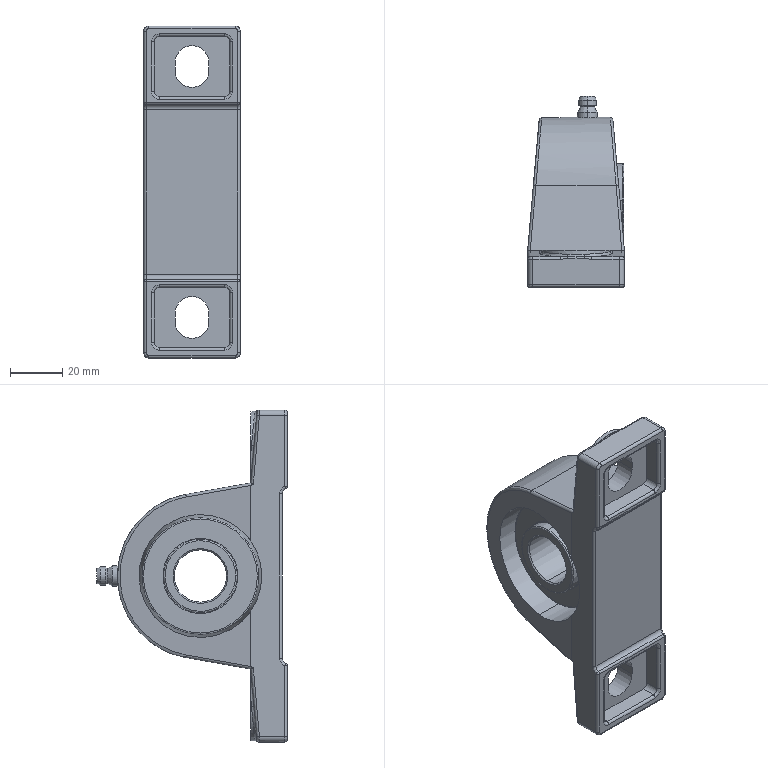Part | STEP file | BRTA-20 pillow block bearing Shanglong | 2 solids | 179 faces | box 37 x 73.015 x 127 mm | volume 112012 mm3 | cylinder 78 | spline 49 | plane 42 | cone 10 | commonest cylinder face diameters 2 x34 4 x14 13 x6 6 x4 28 x4 28.8 x4